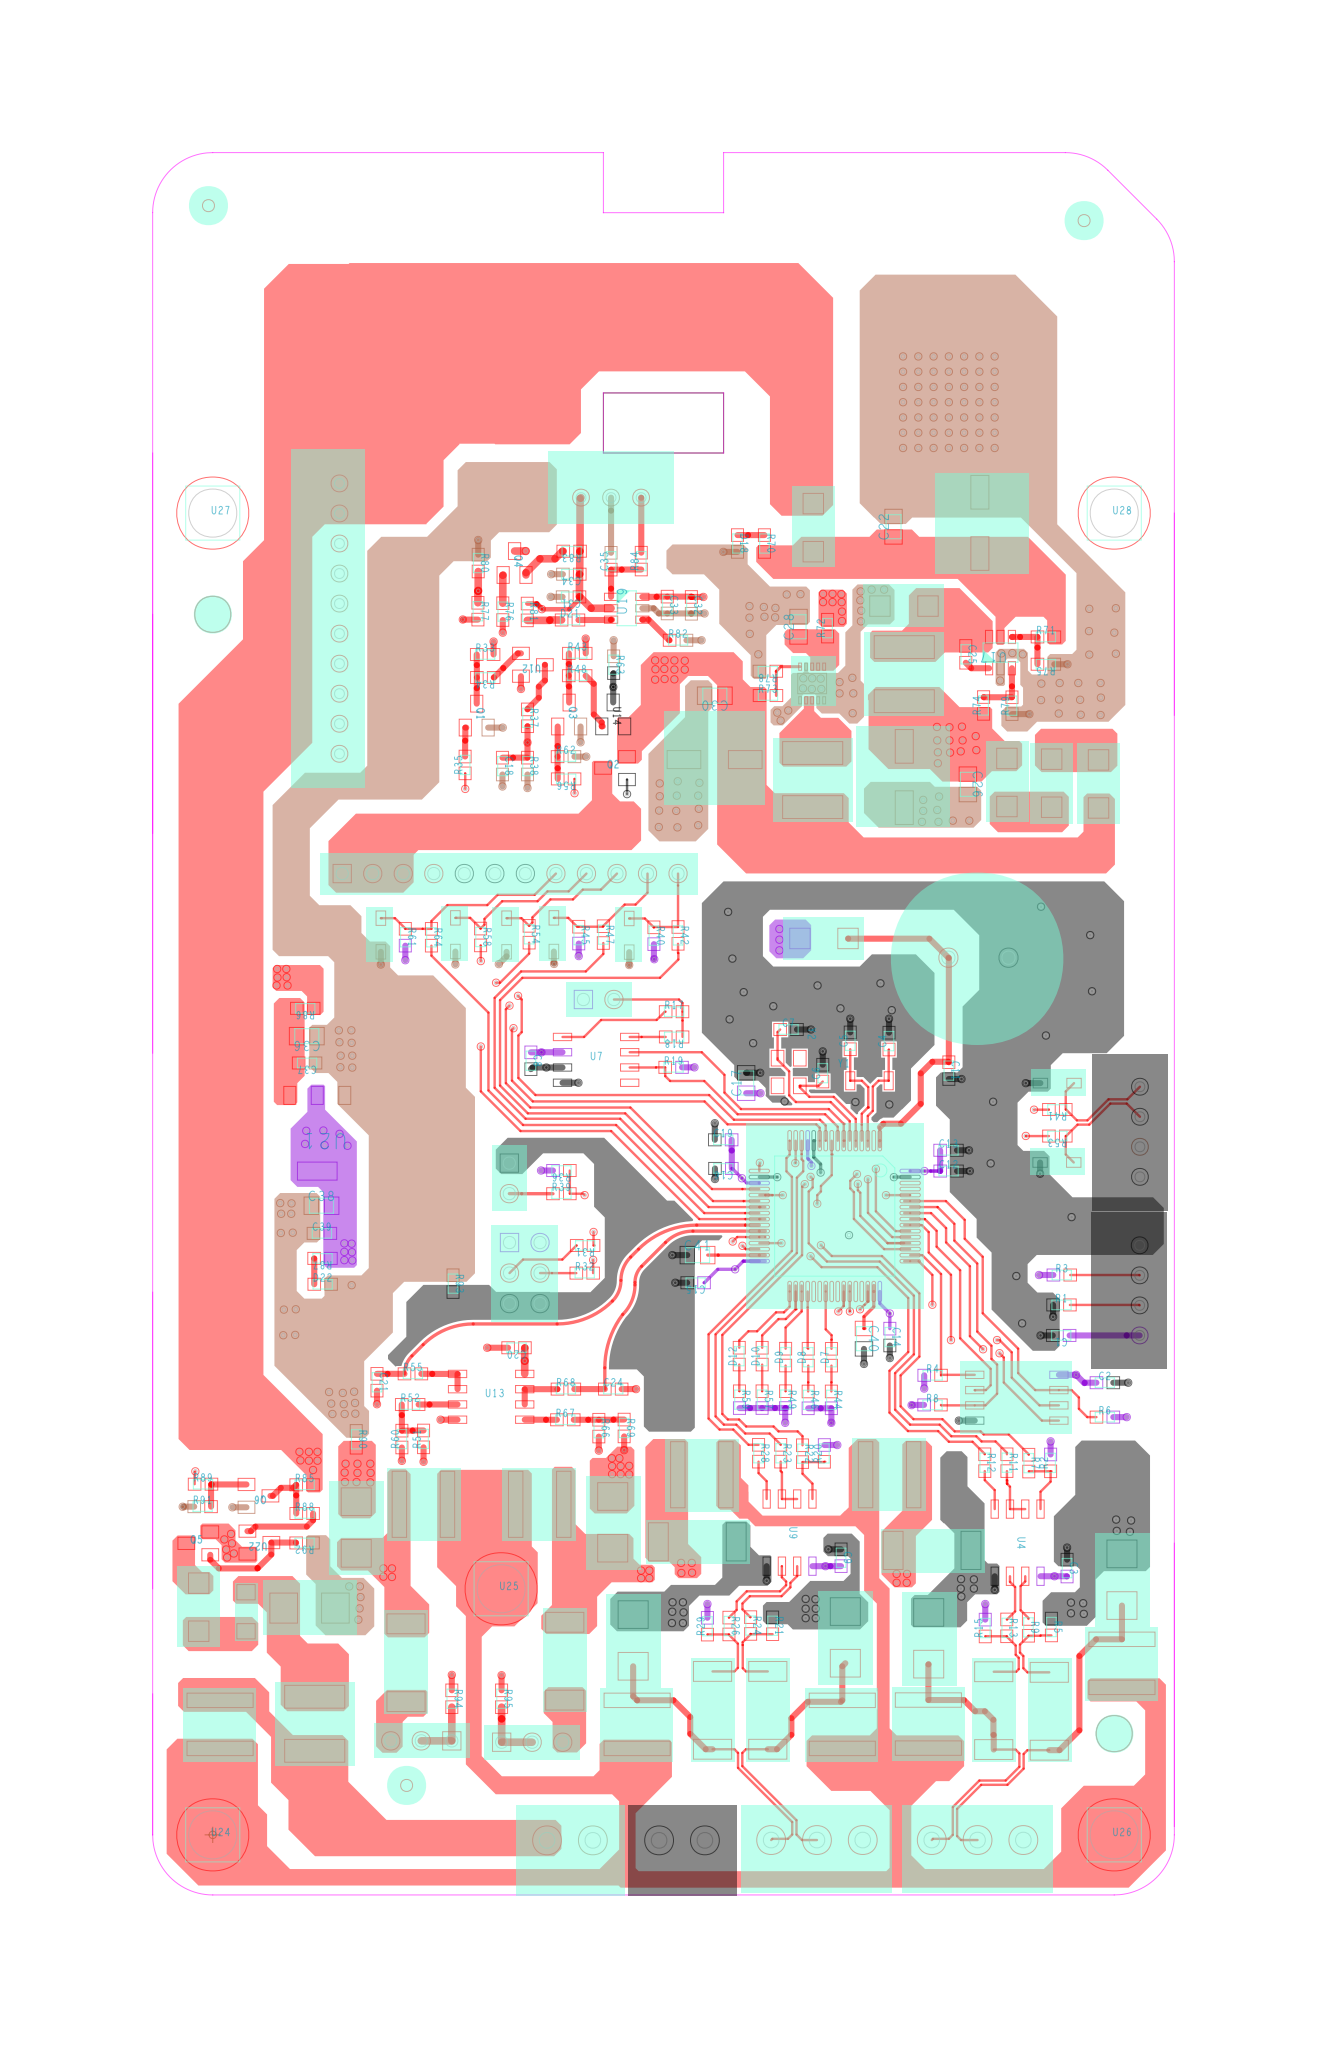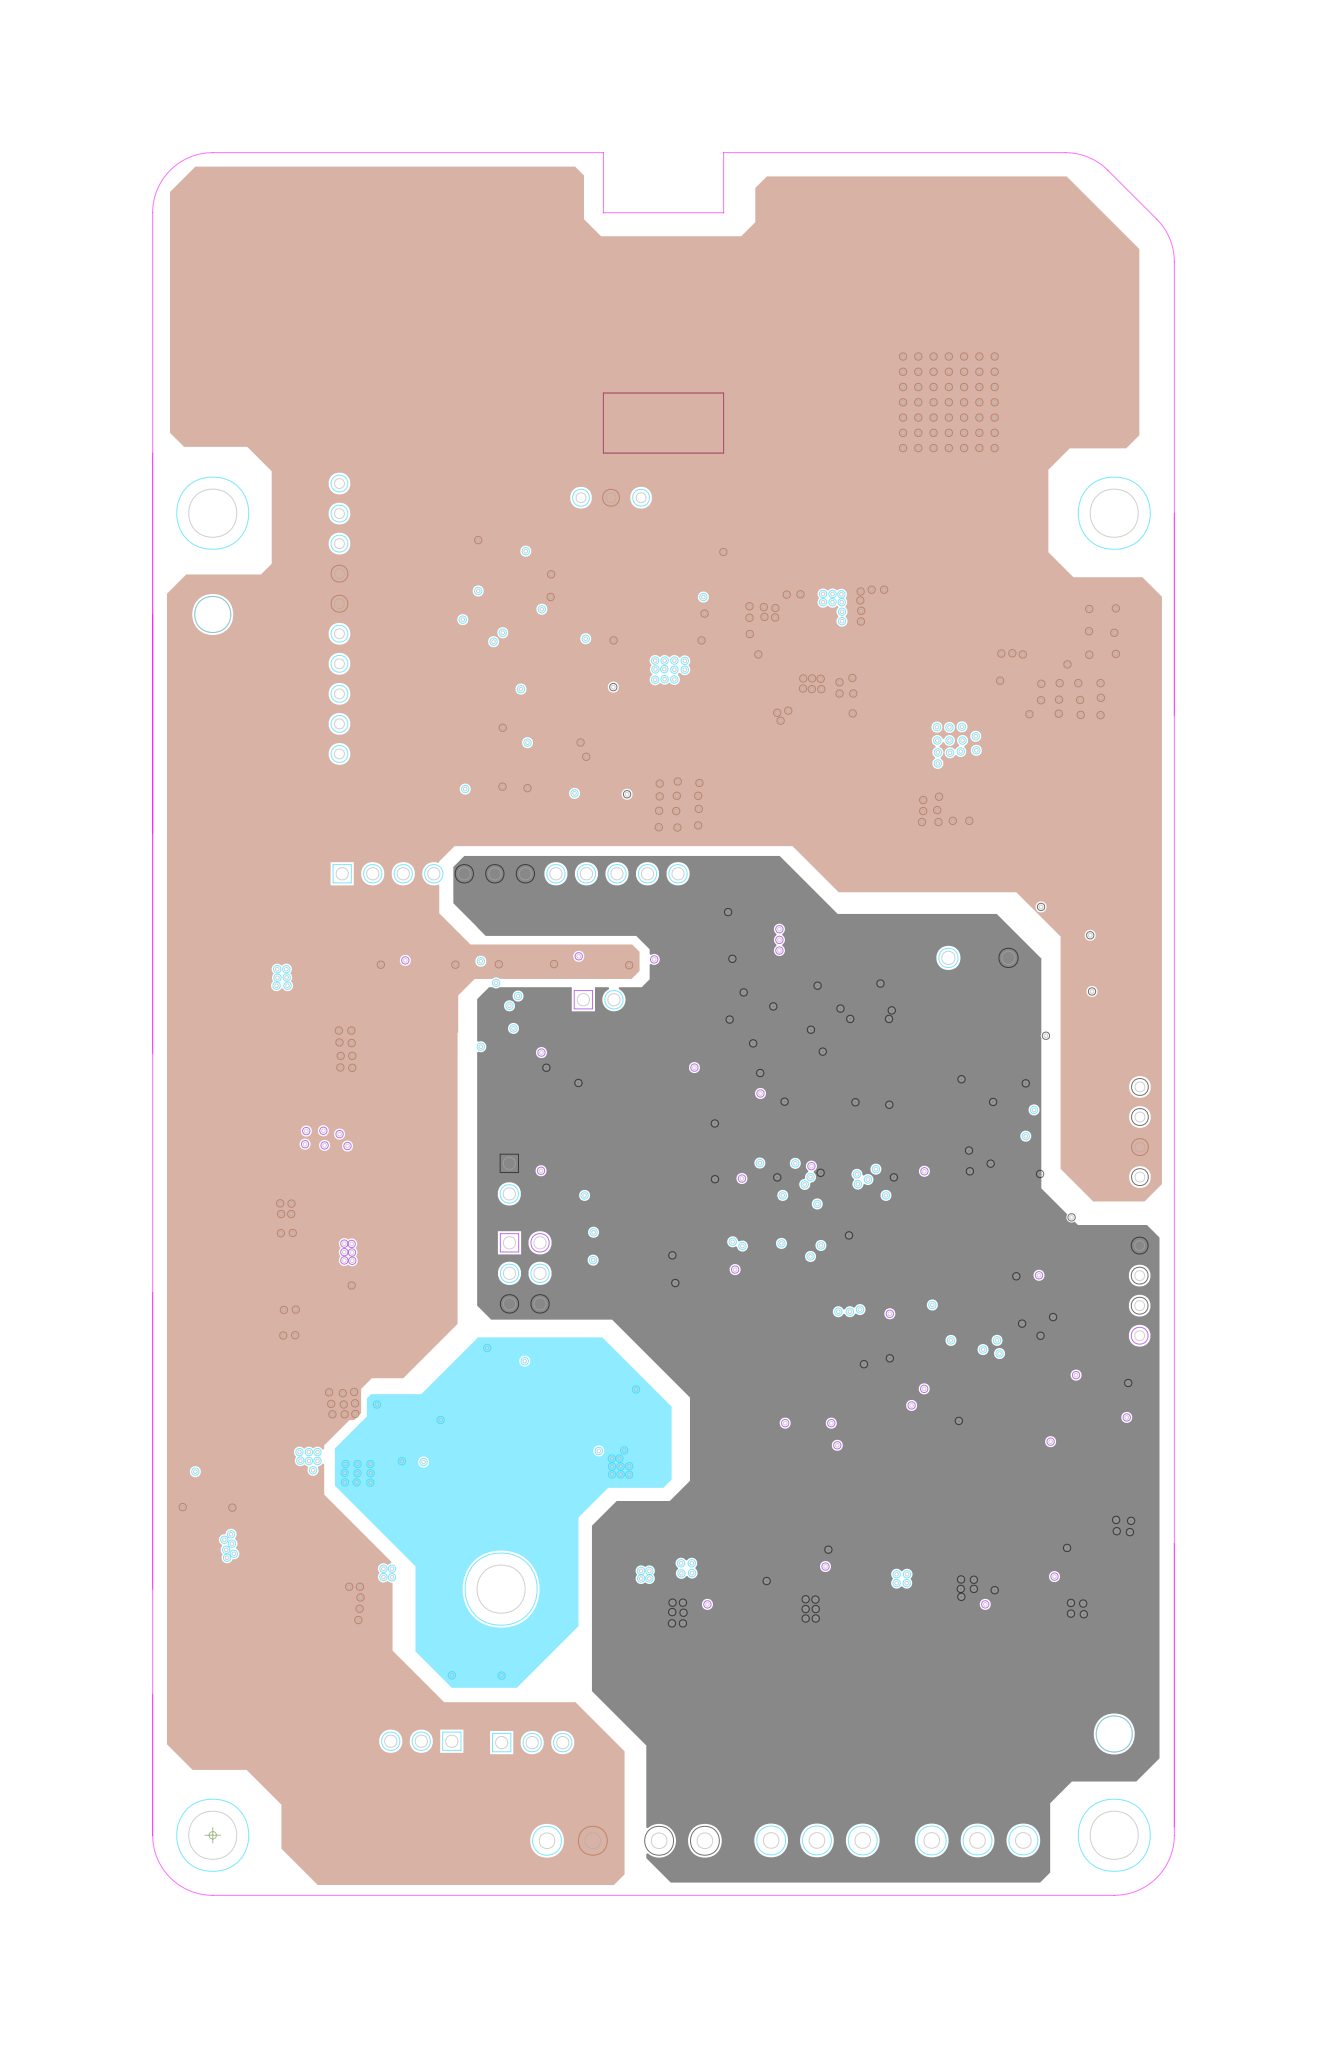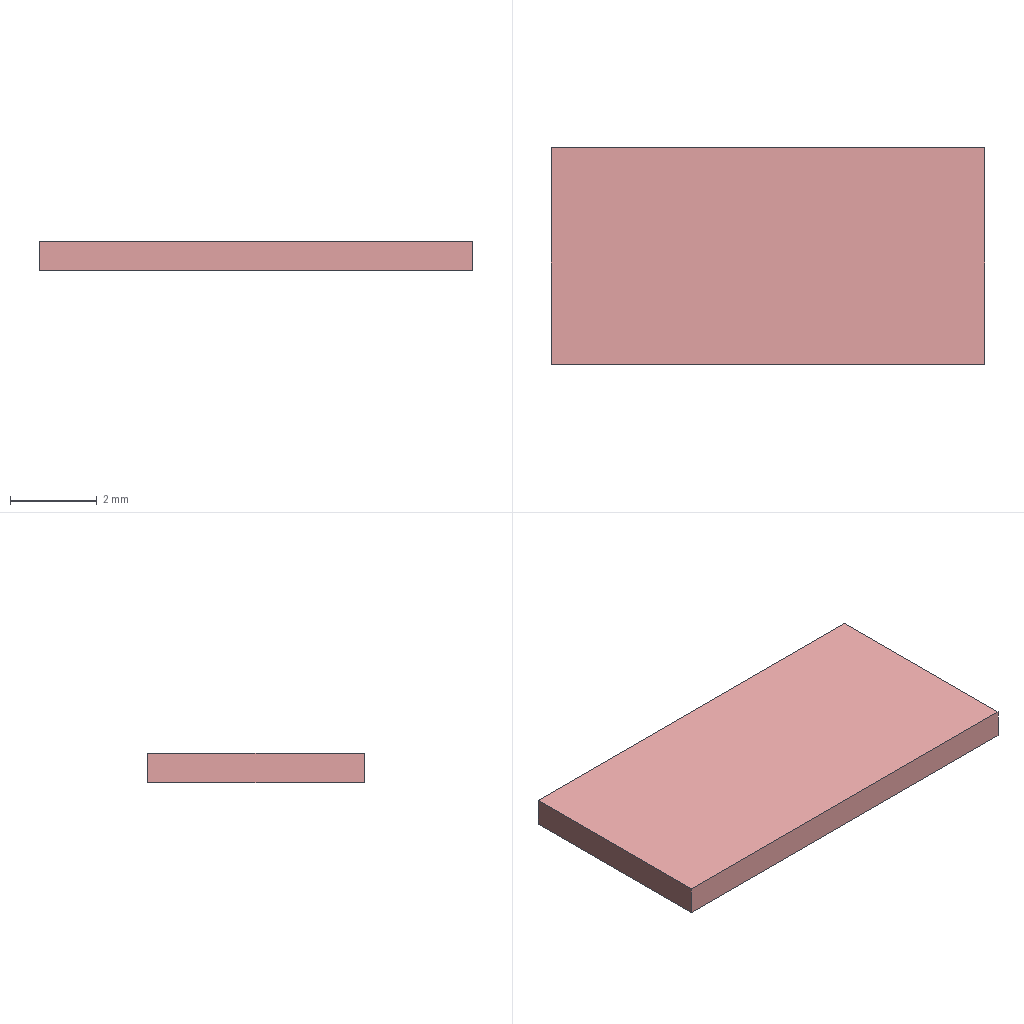Circuit board layout | Cadence Allegro | box 10 x 5 x 0.7 mm
Layer stack:
# Cadence Allegro layer stack of  (unit mm; from the constraint file cross-section; dielectric type: 0 not recorded (Allegro does not mark core vs prepreg), 3 surface material)
index,name,kind,layer,copper_thickness_mm,dielectric_type,dielectric_thickness_mm,dielectric_material,dielectric_constant
0,Top Surface,other,,,,,,
1,TOP,copper,TOP,0.0305,,,,
2,Dielectric1,dielectric,,,0,0.2032,FR-4,4.5
3,GND02,copper,GND02,0.0305,,,,
4,Dielectric2,dielectric,,,0,0.2032,FR-4,4.5
5,PWR03,copper,PWR03,0.0305,,,,
6,Dielectric3,dielectric,,,0,0.2032,FR-4,4.5
7,BOTTOM,copper,BOTTOM,0.0305,,,,
8,Bottom Surface,other,,,,,,
# drill layer pairs: low layer,high layer
drill_pair,TOP,BOTTOM
Part placement:
REFDES,COMP_VALUE,SYM_NAME,SYM_X,SYM_Y,SYM_ROTATE,SYM_MIRROR
C1,104,0603C,2778.984,1636.303,180.000,NO
C2,0.1uF,0603C,2922.020,1481.480,0.000,NO
C3,104,0603C,2798.244,874.031,270.000,NO
C4,22pF,0603C,2215.016,2600.697,90.000,NO
C5,22pF,0603C,2088.016,2601.697,90.000,NO
C6,22pF,0603C,1998.016,2495.697,90.000,NO
C7,22pF,0603C,1886.016,2638.697,0.000,NO
C8,0.1uF,0603C,1042.004,2536.331,270.000,NO
C9,104,0603C,2058.000,908.000,270.000,NO
C10,5.5V/0.47F,FL,2508.000,2874.000,90.000,NO
C11,0.1uF,0603C,2411.000,2504.000,270.000,NO
C12,104,0603C,2410.240,2174.925,0.000,NO
C13,104,0603C,2410.000,2243.000,0.000,NO
C14,104,0603C,2217.717,1630.980,270.000,NO
C15,104,0603C,1581.630,1808.996,180.000,NO
C16,104,0603C,1672.579,2183.469,180.000,NO
C17,2.2uF,0805C,1747.157,2463.398,90.000,NO
C18,0.1uF,0603C,948.925,3501.768,270.000,NO
C19,0.1uF,0603C,1671.984,2277.303,0.000,NO
C20,104,0603C,995.000,1596.000,180.000,NO
C21,104,0603C,537.925,1482.988,270.000,NO
C22,10uF/25V,0805C,2229.819,4286.079,90.000,NO
C23,10uF/25V,F80,2512.614,4298.594,0.000,NO
C24,104,0603C,1311.760,1460.531,0.000,NO
C25,10nF,0603C,2466.480,3867.921,270.000,NO
C26,22uF/10V,0805C,2473.323,3441.937,270.000,NO
C27,10uF/25V,F80,2265.000,3466.000,180.000,NO
C28,22uF,0805C,1918.709,3958.315,90.000,NO
C29,10uF/25V,F80,1643.787,3523.028,90.000,NO
C30,22uF,0805C,1644.429,3732.390,180.000,NO
C31,1uF,0603C,1173.587,4056.232,180.000,NO
C32,0.1uF,0603C,1567.768,4028.409,270.000,NO
C33,1uF,0603C,1488.768,4029.413,270.000,NO
C34,0.1uF,0603C,1174.571,4130.469,180.000,NO
C35,0.1uF,0603C,1304.602,4173.008,90.000,NO
C36,10uF,0805C,308.000,2617.000,180.000,NO
C37,0.1uF,0603C,309.000,2529.000,180.000,NO
C38,10uF,0805C,356.142,2061.291,0.000,NO
C39,0.1uF,0603C,357.492,1970.685,0.000,NO
C40,2.2uF/6.3V,0805C,2133.016,1625.697,270.000,NO
C41,2.2uF/6.3V,0805C,1587.803,1899.524,0.000,NO
D1,SMBJ6.5CA,SMB,2978.000,836.000,270.000,NO
D2,SMBJ6.5CA,SMB,2345.000,644.000,270.000,NO
D3,SMBJ6.5CA,SMB,2072.000,647.000,270.000,NO
D4,30V,SMA,2002.000,2937.000,0.000,NO
D5,SMBJ6.5CA,SMB,1377.000,637.000,270.000,NO
D6,AC,SOD-323,2766.000,2463.000,0.000,NO
D7,LED,LED0603,2026.551,1564.972,90.000,NO
D8,LED,LED0603,1950.551,1565.083,90.000,NO
D9,LED,LED0603,1876.315,1565.303,90.000,NO
D10,LED,LED0603,1799.551,1568.421,90.000,NO
D11,AC,SOD-323,2765.000,2203.000,0.000,NO
D12,LED,LED0603,1724.551,1568.531,90.000,NO
D13,SMBJ15CA,SMB,470.000,1007.000,270.000,NO
D14,SK36,SMA,2264.000,4026.000,0.000,NO
D15,M7,SMA,1967.000,4283.000,270.000,NO
D16,SMBJ15CA,SMB,1310.000,1024.000,270.000,NO
D17,SS36,SMA,2601.244,3448.035,270.000,NO
D18,LED,LED0603,1718.768,4231.071,270.000,NO
D19,SS36,SMA,2747.787,3445.740,90.000,NO
D20,SS36,SMA,2901.244,3443.272,270.000,NO
D21,LED,LED0603,1170.193,3980.449,0.000,NO
D22,LED,LED0603,360.000,1804.000,0.000,NO
D23,M7,SMA,-46.000,746.000,270.000,NO
D24,SMBJ15CA,SMB,317.000,743.000,0.000,NO
D25,AC,SOD323,794.764,2949.346,90.000,NO
D26,AC,SOD323,550.583,2948.346,90.000,NO
D27,AC,SOD323,962.461,2948.346,90.000,NO
D28,AC,SOD323,1117.280,2949.346,90.000,NO
D29,AC,SOD323,1364.098,2947.346,90.000,NO
F1,JK-NSMD010,1206,109.000,731.000,270.000,NO
J1,USB,XR1X4,3036.000,1784.000,90.000,NO
J2,down,DIP2X1,1264.000,2737.000,90.000,NO
J3,BOOT,DIP2X3,1022.016,1840.697,90.000,NO
J4,485_1,KF2EDG-3_81-3-V,2505.000,-17.000,180.000,NO
J5,485_2,KF2EDG-3_81-3-V,1979.000,-17.000,180.000,NO
J6,CON2,KF2EDG-3_81-2-V,1170.000,-18.000,180.000,NO
J7,CON2,KF2EDG-3_81-2-V,1537.000,-18.000,180.000,NO
J8,SYS_RST,DIP2X1,971.346,2150.925,0.000,NO
J9,CON10,XR1X10,415.000,3985.000,90.000,NO
J10,USB,XR1X4,3036.890,2303.563,90.000,NO
J11,CON12,DIP1X12,974.016,3149.606,90.000,NO
J12,JUM1,DIP1X3,1046.323,303.583,90.000,NO
J13,JUM2,DIP1X3,683.000,308.000,270.000,NO
L1,SLF7032T-6R8M1R6-2PF,6045,2265.000,3803.000,270.000,NO
L2,INDUCTOR,6045,1965.000,3456.000,270.000,NO
L3,SMTDR32-560M,6045,334.000,364.000,90.000,NO
Q1,NPN,SOT-23,864.531,3666.685,270.000,NO
Q2,PMOS-3P,SOT-23,1318.000,3495.000,0.000,NO
Q3,NPN,SOT-23,1167.240,3670.295,270.000,NO
Q4,PMOS-3P,SOT-23,988.531,4166.685,270.000,NO
Q5,PMOS-3P,SOT-23,-47.000,955.000,0.000,NO
Q6,NPN,SOT-23,149.295,1110.760,180.000,NO
R1,10k,0603R,2779.984,1736.303,0.000,NO
R2,4.7k,0603R,2744.315,1218.780,90.000,NO
R3,10k,0603R,2780.984,1834.303,0.000,NO
R4,10k,0603R,2357.866,1505.717,0.000,NO
R5,4.7k,0603R,2747.000,681.000,270.000,NO
R6,10k,0603R,2922.087,1368.717,0.000,NO
R7,330,0603R,2672.717,1217.945,270.000,NO
R8,10k,0603R,2357.528,1408.717,0.000,NO
R9,330,0603R,2671.717,679.835,270.000,NO
R10,5.1/2W,2512,2740.000,405.000,270.000,NO
R11,330,0603R,2601.244,1219.370,270.000,NO
R12,330,0603R,2528.717,1219.374,270.000,NO
R13,330,0603R,2600.717,678.264,270.000,NO
R14,5.1/2W,2512,2558.000,407.000,270.000,NO
R15,4.7k,0603R,2530.315,677.669,90.000,NO
R16,5.1/2W,2512,2356.000,932.000,180.000,NO
R17,2k,0603R,1511.000,2697.000,0.000,NO
R18,2k,0603R,1511.228,2614.315,180.000,NO
R19,2k,0603R,1509.488,2514.717,0.000,NO
R20,4.7k,0603R,2003.315,1249.780,90.000,NO
R21,4.7k,0603R,1833.717,685.063,270.000,NO
R22,330,0603R,1931.717,1248.945,270.000,NO
R23,330,0603R,1860.244,1250.370,270.000,NO
R24,330,0603R,1761.717,685.835,270.000,NO
R25,5.1/2W,2512,1818.000,408.000,270.000,NO
R26,330,0603R,1690.717,684.264,270.000,NO
R27,5.1/2W,2512,1637.000,408.000,270.000,NO
R28,330,0603R,1787.717,1250.374,270.000,NO
R29,4.7k,0603R,1620.315,683.669,90.000,NO
R30,5.1/2W,2512,1587.000,960.000,180.000,NO
R31,100k,0603R,1219.720,1931.075,180.000,NO
R32,100k,0603R,1218.358,1840.531,0.000,NO
R33,10k,0603R,892.248,3867.398,0.000,NO
R34,10k,0603R,892.673,3791.996,180.000,NO
R35,4.7k,0603R,826.602,3505.539,90.000,NO
R36,10k,0603R,1142.016,2176.697,180.000,NO
R37,12k,0603R,1030.925,3659.949,270.000,NO
R38,30k,0603R,1030.925,3501.839,270.000,NO
R39,330,0603R,1142.016,2100.697,0.000,NO
R40,100k,0603R,1445.000,2946.000,270.000,NO
R41,RES2,0603R,2766.350,2376.531,180.000,NO
R42,330,0603R,1524.000,2947.000,270.000,NO
R43,1k,0603R,1194.000,3871.000,0.000,NO
R44,2k,0603R,2026.244,1425.311,270.000,NO
R45,100k,0603R,1198.756,2947.898,270.000,NO
R46,2k,0603R,1950.244,1425.201,270.000,NO
R47,330,0603R,1279.283,2949.618,270.000,NO
R48,1k,0603R,1193.713,3797.925,0.000,NO
R49,2k,0603R,1876.244,1426.091,270.000,NO
R50,5.1/2W,2512,633.000,564.000,270.000,NO
R51,91k/1%,0603R,690.469,1297.339,90.000,NO
R52,10k,0603R,646.657,1410.004,0.000,NO
R53,RES2,0603R,2766.461,2289.531,180.000,NO
R54,330,0603R,1036.283,2950.728,270.000,NO
R55,100,0603R,655.559,1510.531,0.000,NO
R56,1k,0603R,1157.496,3459.787,180.000,NO
R57,2k,0603R,1799.244,1425.980,270.000,NO
R58,330,0603R,877.283,2941.839,270.000,NO
R59,2k,0603R,1725.244,1425.870,270.000,NO
R60,30k/1%,0603R,619.469,1296.780,90.000,NO
R61,100k,0603R,630.756,2941.008,270.000,NO
R62,4.7k,0603R,1157.047,3532.717,0.000,NO
R63,100k,0603R,1313.000,3834.000,270.000,NO
R64,330,0603R,716.283,2940.949,270.000,NO
R65,5.1/2W,2512,1153.000,569.000,270.000,NO
R66,91k/1%,0603R,1264.531,1332.551,270.000,NO
R67,10k,0603R,1154.878,1360.004,0.000,NO
R68,100,0603R,1156.669,1460.531,0.000,NO
R69,30k/1%,0603R,1347.531,1333.110,270.000,NO
R70,10k,0603R,1807.004,4231.012,270.000,NO
R71,100k,0603R,2728.941,3924.925,0.000,NO
R72,0,0603R,2013.787,3953.713,90.000,NO
R73,536k/1%,0603R,1818.583,3732.925,0.000,NO
R74,49.9k/1%,0603R,2524.787,3700.374,90.000,NO
R75,30k,0603R,2728.760,3835.469,180.000,NO
R76,10k,0603R,950.004,4007.902,270.000,NO
R77,2.74K/1%,0603R,868.531,4009.228,270.000,NO
R78,100k/1%,0603R,1818.118,3812.469,180.000,NO
R79,9.53k/1%,0603R,2617.787,3699.701,90.000,NO
R80,4.7K/1%,0603R,869.531,4166.902,270.000,NO
R81,2k,0603R,1030.244,4006.760,270.000,NO
R82,2k,0603R,1524.000,3914.000,0.000,NO
R83,0,0603R,1175.571,4205.756,180.000,NO
R84,10k,0603R,1403.602,4173.350,90.000,NO
R85,1k,0603R,300.933,1146.925,0.000,NO
R86,0,0603R,303.000,2708.000,180.000,NO
R87,2k,0603R,359.539,1888.756,180.000,NO
R88,1k,0603R,301.043,1052.925,0.000,NO
R89,1k,0603R,-31.850,1148.925,0.000,NO
R90,0,0603R,470.000,1296.000,270.000,NO
R91,4.7k,0603R,-33.130,1075.398,0.000,NO
R92,1k,0603R,300.772,956.469,180.000,NO
R93,0,0603R,787.000,1806.000,270.000,NO
R94,249/1%,0603R,783.000,446.000,270.000,NO
R95,249/1%,0603R,946.000,446.000,270.000,NO
U1,STM32F205,LQFP-64,2037.244,2027.366,270.000,NO
U2,25Q32VSIG,SOIC-8_208,2633.634,1432.244,0.000,NO
U3,470M,SMD5050,2978.000,562.000,270.000,NO
U4,SP3485E,SO8,2711.244,1067.366,270.000,NO
U5,470M,SMD5050,2344.000,363.000,270.000,NO
U6,470M,SMD5050,2217.000,1180.000,180.000,NO
U7,MAX706R,SO8,1145.634,2614.244,0.000,NO
U8,470M,SMD5050,2062.000,362.000,270.000,NO
U9,SP3485E,SO8,1964.244,1100.366,270.000,NO
U10,470M,SMD5050,1602.000,1180.000,0.000,NO
U11,470M,SMD5050,1390.000,362.000,270.000,NO
U12,PNP,SOT-23,1048.295,3833.760,180.000,NO
U13,LM2904,SO8,801.854,1510.240,0.000,NO
U14,PNP,SOT-23,1311.531,3670.685,270.000,NO
U15,470M,SMD5050,690.000,1083.000,0.000,NO
U16,470M,SMD5050,1071.000,1083.000,180.000,NO
U17,MP2359DJ,SOT23-6,2580.181,3873.598,90.000,NO
U18,SGM6014ADJ,TDFN-3X3-10L,1963.244,3772.366,270.000,NO
U19,BQ21040,SOT23-6,1355.850,4018.850,0.000,NO
U20,BAT,XR1X3,1304.618,4381.417,0.000,NO
U21,TLV1117LV,SOT-223,432.366,2422.756,180.000,NO
U22,PNP,SOT-23,152.295,957.760,180.000,NO
U23,470M,SMD5050,24.000,362.000,270.000,NO
U24,TEST POINT A,HOLE,0.000,0.000,0.000,NO
U25,TEST POINT A,HOLE,944.531,806.287,0.000,NO
U26,TEST POINT A,HOLE,2952.756,0.000,0.000,NO
U27,TEST POINT A,HOLE,0.000,4330.709,0.000,NO
U28,TEST POINT A,HOLE,2952.756,4330.709,0.000,NO
Y1,8M,XTAL3215,2088.016,2470.697,0.000,NO
Y2,32.768K,XTAL3225,1850.016,2544.697,270.000,NO
Pad and via stacks:
# Allegro (Cadence) via spans and padstacks; design units: ("mils" 3 1000)
# via spans: padstack,start_layer,end_layer,net_example,count
VIA12_24,ETCH/TOP,ETCH/BOTTOM,VCC_12V,435
# Allegro padstack definitions: name,start_layer,end_layer,drill,plating,holeType,type
VIA30D16,"ETCH/TOP","ETCH/BOTTOM",16.0,"PLATED","circle_drill","through"
R180_160,"ETCH/TOP","ETCH/TOP",0.0,"PLATED","none","smd"
PTH_C472D276S40,"ETCH/TOP","ETCH/BOTTOM",27.559,"PLATED","circle_drill","through"
PTH_S472D276S40,"ETCH/TOP","ETCH/BOTTOM",27.559,"PLATED","circle_drill","through"
RE118_11X98_43,"ETCH/TOP","ETCH/TOP",0.0,"NON_PLATED","none","smd"
C43_31D43_31,"ETCH/TOP","ETCH/BOTTOM",43.311,"PLATED","circle_drill","through"
R105_100,"ETCH/TOP","ETCH/TOP",0.0,"PLATED","none","smd"
R170_135,"ETCH/TOP","ETCH/TOP",0.0,"PLATED","none","smd"
R145_120,"ETCH/TOP","ETCH/TOP",0.0,"PLATED","none","smd"
RE350X100,"ETCH/TOP","ETCH/TOP",0.0,"PLATED","none","smd"
RE55X40,"ETCH/TOP","ETCH/TOP",0.0,"NON_PLATED","none","smd"
R225_160,"ETCH/TOP","ETCH/TOP",0.0,"PLATED","none","smd"
S210,"ETCH/TOP","ETCH/TOP",0.0,"PLATED","none","smd"
RE90X95,"ETCH/TOP","ETCH/TOP",0.0,"NON_PLATED","none","smd"
SMD_R787X1181P0S40,"ETCH/TOP","ETCH/TOP",0.0,"PLATED","none","smd"
SMD_R98X472P0S40,"ETCH/TOP","ETCH/TOP",0.0,"PLATED","none","smd"
S220H120T220_240_40,"ETCH/TOP","ETCH/BOTTOM",47.244,"PLATED","circle_drill","through"
C220H120T220_240_40,"ETCH/TOP","ETCH/BOTTOM",47.244,"PLATED","circle_drill","through"
S160H105T155_190_40,"ETCH/TOP","ETCH/BOTTOM",41.339,"PLATED","circle_drill","through"
C160H105T155_190_40,"ETCH/TOP","ETCH/BOTTOM",41.339,"PLATED","circle_drill","through"
SMD_R472X709P0S40,"ETCH/TOP","ETCH/TOP",0.0,"PLATED","none","smd"
SMD_R276X709P0S40,"ETCH/TOP","ETCH/TOP",0.0,"PLATED","none","smd"
SMD_R591X1102P0S40,"ETCH/TOP","ETCH/TOP",0.0,"PLATED","none","smd"
SMD_R433X709P0S40,"ETCH/TOP","ETCH/TOP",0.0,"PLATED","none","smd"
PTH_O1800X800SLOT500X1100S40,"ETCH/TOP","ETCH/BOTTOM",50.0,"PLATED","oval slot","through"
PTH_O800X1800SLOT500X1200S40,"ETCH/TOP","ETCH/BOTTOM",50.0,"PLATED","oval slot","through"
PTH_O800X1800SLOT500X1100S40,"ETCH/TOP","ETCH/BOTTOM",50.0,"PLATED","oval slot","through"
PTH_S630D362S40,"ETCH/TOP","ETCH/BOTTOM",36.22,"PLATED","circle_drill","through"
PTH_C630D362S40,"ETCH/TOP","ETCH/BOTTOM",36.22,"PLATED","circle_drill","through"
PTH_C1496D906S40,"ETCH/TOP","ETCH/BOTTOM",90.551,"PLATED","circle_drill","through"
SMD_R984X787P0S40,"ETCH/TOP","ETCH/TOP",0.0,"PLATED","none","smd"
SMD_R236X787P0S40,"ETCH/TOP","ETCH/TOP",0.0,"PLATED","none","smd"
S140H80,"ETCH/TOP","ETCH/BOTTOM",31.496,"PLATED","circle_drill","through"
C140H80,"ETCH/TOP","ETCH/BOTTOM",31.496,"PLATED","circle_drill","through"
S140H90T140_170_40,"ETCH/TOP","ETCH/BOTTOM",35.433,"PLATED","circle_drill","through"
C140H90T140_170_40,"ETCH/TOP","ETCH/BOTTOM",35.433,"PLATED","circle_drill","through"
C355H235T285_330_50,"ETCH/TOP","ETCH/BOTTOM",92.52,"PLATED","circle_drill","through"
PTH_C591D402S40,"ETCH/TOP","ETCH/BOTTOM",40.161,"PLATED","circle_drill","through"
PTH_C600D350S40,"ETCH/TOP","ETCH/BOTTOM",35.0,"PLATED","circle_drill","through"
PTH_C866D650S40,"ETCH/TOP","ETCH/BOTTOM",64.961,"PLATED","circle_drill","through"
PTH_S600D350S40,"ETCH/TOP","ETCH/BOTTOM",35.0,"PLATED","circle_drill","through"
RE200X125,"ETCH/TOP","ETCH/TOP",0.0,"PLATED","none","smd"
RE75X40,"ETCH/TOP","ETCH/TOP",0.0,"NON_PLATED","none","smd"
SQ120,"ETCH/TOP","ETCH/TOP",0.0,"PLATED","none","smd"
RE620X580,"ETCH/TOP","ETCH/TOP",0.0,"NON_PLATED","none","smd"
RE300X160,"ETCH/TOP","ETCH/TOP",0.0,"NON_PLATED","none","smd"
C100H60,"ETCH/TOP","ETCH/BOTTOM",23.622,"PLATED","circle_drill","through"
RE100H60,"ETCH/TOP","ETCH/BOTTOM",23.622,"PLATED","circle_drill","through"
R105_45,"ETCH/TOP","ETCH/TOP",0.0,"PLATED","none","smd"
RE65X180,"ETCH/TOP","ETCH/TOP",0.0,"PLATED","none","smd"
H70,"ETCH/TOP","ETCH/BOTTOM",27.559,"PLATED","circle_drill","through"
SMD_R100X650P0S40,"ETCH/TOP","ETCH/TOP",0.0,"PLATED","none","smd"
RE150X80,"ETCH/TOP","ETCH/TOP",0.0,"NON_PLATED","none","smd"
SMD_R512X413P0S40,"ETCH/TOP","ETCH/TOP",0.0,"PLATED","none","smd"
RE60X24,"ETCH/TOP","ETCH/TOP",0.0,"NON_PLATED","none","smd"
RE43_31X19_68,"ETCH/TOP","ETCH/TOP",0.0,"PLATED","none","smd"
RE134X170,"ETCH/TOP","ETCH/TOP",0.0,"PLATED","none","smd"
R110_60,"ETCH/TOP","ETCH/TOP",0.0,"PLATED","none","smd"
RE100X150,"ETCH/TOP","ETCH/TOP",0.0,"PLATED","none","smd"
RE330X150,"ETCH/TOP","ETCH/TOP",0.0,"PLATED","none","smd"
RE39_37X11_81,"ETCH/TOP","ETCH/TOP",0.0,"NON_PLATED","none","smd"
RE11_81X39_37,"ETCH/TOP","ETCH/TOP",0.0,"NON_PLATED","none","smd"
SQ124,"ETCH/TOP","ETCH/TOP",0.0,"NON_PLATED","none","smd"
SQ20,"ETCH/TOP","ETCH/TOP",0.0,"NON_PLATED","none","smd"
R155_60,"ETCH/TOP","ETCH/TOP",0.0,"PLATED","none","smd"
SMD_R118X315P0S40,"ETCH/TOP","ETCH/TOP",0.0,"PLATED","none","smd"
R27X39,"ETCH/TOP","ETCH/TOP",0.0,"PLATED","none","smd"
SMD_R98X315P0S40,"ETCH/TOP","ETCH/TOP",0.0,"PLATED","none","smd"
SMD_S984P0S40,"ETCH/TOP","ETCH/TOP",0.0,"PLATED","none","smd"
SMD_R591X295P0S40,"ETCH/TOP","ETCH/TOP",0.0,"PLATED","none","smd"
SMD_R295X591P0S40,"ETCH/TOP","ETCH/TOP",0.0,"PLATED","none","smd"
PTH_C600D300S40,"ETCH/TOP","ETCH/BOTTOM",30.0,"PLATED","circle_drill","through"
C177_17D137_80,"ETCH/TOP","ETCH/BOTTOM",157.48,"PLATED","circle_drill","through"
B160_60,"ETCH/TOP","ETCH/TOP",0.0,"PLATED","none","smd"
PTH_O1024X709SLOT394X630S40,"ETCH/TOP","ETCH/BOTTOM",39.37,"PLATED","oval slot","through"
VIA12_24,"ETCH/TOP","ETCH/BOTTOM",12.0,"PLATED","circle_drill","through"
Y300,"ETCH/TOP","ETCH/BOTTOM",118.11,"NON_PLATED","circle_drill","through"
C83D53,"ETCH/TOP","ETCH/BOTTOM",53.0,"PLATED","circle_drill","through"
R18X20,"ETCH/TOP","ETCH/TOP",0.0,"NON_PLATED","none","smd"
Y3,"ETCH/TOP","ETCH/TOP",0.0,"PLATED","none","smd"
SMD_OV65X12,"ETCH/TOP","ETCH/TOP",0.0,"PLATED","none","smd"
F15,"ETCH/TOP","ETCH/BOTTOM",40.0,"PLATED","circle_drill","through"
F152,"ETCH/TOP","ETCH/BOTTOM",40.0,"PLATED","circle_drill","through"
R23X25,"ETCH/TOP","ETCH/TOP",0.0,"NON_PLATED","none","smd"
S17,"ETCH/TOP","ETCH/TOP",0.0,"NON_PLATED","none","smd"
R12X8,"ETCH/TOP","ETCH/TOP",0.0,"NON_PLATED","none","smd"
R127X152,"ETCH/TOP","ETCH/TOP",0.0,"NON_PLATED","none","smd"
R50X30,"ETCH/TOP","ETCH/TOP",0.0,"NON_PLATED","none","smd"
R35X16,"ETCH/TOP","ETCH/TOP",0.0,"PLATED","none","smd"
Y6T,"ETCH/TOP","ETCH/BOTTOM",43.307,"PLATED","circle_drill","through"
Y8T,"ETCH/TOP","ETCH/BOTTOM",32.283,"PLATED","circle_drill","through"
R15X28,"ETCH/TOP","ETCH/TOP",0.0,"NON_PLATED","none","smd"
Y24,"ETCH/TOP","ETCH/BOTTOM",51.181,"PLATED","circle_drill","through"
R60X24,"ETCH/TOP","ETCH/TOP",0.0,"PLATED","none","smd"
R170X240,"ETCH/TOP","ETCH/TOP",0.0,"PLATED","none","smd"
D3,"ETCH/TOP","ETCH/BOTTOM",118.11,"NON_PLATED","circle_drill","through"
R550X120,"ETCH/TOP","ETCH/TOP",0.0,"PLATED","none","smd"
R500X190,"ETCH/TOP","ETCH/TOP",0.0,"PLATED","none","smd"
R165X317,"ETCH/TOP","ETCH/TOP",0.0,"NON_PLATED","none","smd"
Design rules, without the lines most boards share, first 13 of 25 lines:
# Cadence Allegro design rules of  (from the Constraint Manager export constraints.dcfx, design unit mil; typed fields in mm)
# columns: name | kind | enabled | priority | scope1 | scope2 | descriptor | typed fields (field=value)
# Allegro precedence (priority 1 wins): 1 Region class-to-class, 2 Region class, 3 Region, 4 class-to-class, 5 DiffPair/Bus/NetGroup override, 6 NetClass, 7 constraint set (CSet) default
# per-layer values are written LAYER=value in the descriptor and LAYER:mm in the typed field; a maximum of 0 means no limit set
# --- net classes (and buses / net groups) ---
# (no net classes defined: every net uses the default constraint sets)
# --- track widths, neck and differential-pair gap (physical constraint sets) ---
DEFAULT | PhysicalCSet | enabled | 7 | Design default | All | Physical Constraint (Min Line Width=8mil) (Max Line Width=100mil) (Min Neck Width=6mil) (Max Neck Length=6mil) (DiffPair Primary Gap=6mil) (DiffPair Neck Gap=6mil) (DiffPair Min Space=6mil) (DiffPair Coupled +Tol=6mil) (DiffPair Coupled -Tol=6mil) (Min BB Via Stagger=6mil) (Max BB Via Stagger=6mil) (T-junctions=ANYWHERE) (Pad-pad direct connect=ALL_ALLOWED) (Allowed vias=VIA12_24) | min_line_width=0.2032 min_neck_width=0.1524 min_bvia_stagger=0.1524 max_bvia_stagger=0.1524 ts_allowed=ANYWHERE diffp_primary_gap=0.1524 diffp_neck_gap=0.1524 max_line_width=2.54 maximum_neck_length=0.1524 pad_pad_direct_connect=ALL_ALLOWED allow_on_etch_subclass=TRUE diffp_coupled_plus=0.1524 diffp_coupled_minus=0.1524 diffp_min_space=0.1524 vias=VIA12_24
# --- clearances: line / pad / via / shape / hole (spacing constraint sets) ---
DEFAULT | SpacingCSet | enabled | 7 | Design default | All | Clearance Constraint (Line-Line=6mil) (Line-SMD Pad=8mil) (Line-Thru Pin=8mil) (Line-Via=8mil) (Line-Shape=8mil) (SMD Pad-SMD Pad=7mil) (Thru Pin-Thru Pin=8mil) (Thru Pin-SMD Pad=7mil) (SMD Pad-Via=8mil) (Thru Pin-Via=8mil) (Via-Via=6mil) (Shape-SMD Pad=6mil) (Shape-Thru Pin=8mil) (Shape-Via=6mil) (Shape-Shape=6mil) (Hole-Hole=8mil) (Hole-Line=8mil) (Hole-Shape=8mil) (BB Via-BB Via=6mil) (uVia-uVia=5mil) | thrupin_to_thrupin_spacing=0.2032 thrupin_to_smdpin_spacing=0.1778 thrupin_to_thruvia_spacing=0.2032 line_to_thrupin_spacing=0.2032 thrupin_to_shape_spacing=0.2032 smdpin_to_smdpin_spacing=0.1778 smdpin_to_thruvia_spacing=0.2032 line_to_smdpin_spacing=0.2032 shape_to_smdpin_spacing=0.1524 thruvia_to_thruvia_spacing=0.1524 line_to_thruvia_spacing=0.2032 shape_to_thruvia_spacing=0.1524 line_to_line_spacing=0.1524 line_to_shape_spacing=0.2032 shape_to_shape_spacing=0.1524 bbv_to_bbv_spacing=0.1524 bbv_to_thrupin_spacing=0.2032 bbv_to_smdpin_spacing=0.2032 bbv_to_thruvia_spacing=0.1524 bbv_to_line_spacing=0.2032 bbv_to_shape_spacing=0.1524 bbv_to_testpin_spacing=0.1524 bbv_to_testvia_spacing=0.1524 testpin_to_testpin_spacing=0.1778 testpin_to_thrupin_spacing=0.2032 smdpin_to_testpin_spacing=0.2032 testpin_to_thruvia_spacing=0.1524 testpin_to_testvia_spacing=0.1524 line_to_testpin_spacing=0.2032 shape_to_testpin_spacing=0.1524 testvia_to_testvia_spacing=0.127 testvia_to_thrupin_spacing=0.2032 smdpin_to_testvia_spacing=0.2032 testvia_to_thruvia_spacing=0.1524 line_to_testvia_spacing=0.2032 shape_to_testvia_spacing=0.1524 bondpad_to_bondpad_spacing=0.127 thrupin_to_bondpad_spacing=0.2032 smdpin_to_bondpad_spacing=0.1524 bondpad_to_thruvia_spacing=0.1524 bondpad_to_line_spacing=0.2032 bondpad_to_shape_spacing=0.1524 bondpad_to_bbv_spacing=0.1524 bondpad_to_testpin_spacing=0.1524 bondpad_to_testvia_spacing=0.127 min_bvia_gap=0.127 hole_to_pin_spacing=0.2032 hole_to_via_spacing=0.2032 hole_to_line_spacing=0.2032 hole_to_shape_spacing=0.2032 hole_to_hole_spacing=0.2032 mvia_to_mvia_spacing=0.127 mvia_to_thrupin_spacing=0.2032 mvia_to_smdpin_spacing=0.2032 mvia_to_thruvia_spacing=0.127 mvia_to_bbv_spacing=0.127 mvia_to_line_spacing=0.2032 mvia_to_shape_spacing=0.127 mvia_to_testpin_spacing=0.127 mvia_to_testvia_spacing=0.127 bondpad_to_mvia_spacing=0.127 bondpad_to_bondpad_diffp_spc=0.127
DEFAULT | SameNetSpacingCSet | enabled | 7 | Design default | All | Same-Net Clearance (Line-Line=5mil) (Line-SMD Pad=5mil) (Line-Thru Pin=5mil) (Line-Via=5mil) (Line-Shape=5mil) (SMD Pad-SMD Pad=5mil) (Thru Pin-Thru Pin=5mil) (Thru Pin-SMD Pad=5mil) (SMD Pad-Via=5mil) (Thru Pin-Via=5mil) (Via-Via=5mil) (Shape-SMD Pad=5mil) (Shape-Thru Pin=5mil) (Shape-Via=5mil) (Shape-Shape=5mil) (Hole-Hole=8mil) (Hole-Line=8mil) (Hole-Shape=8mil) (BB Via-BB Via=5mil) (uVia-uVia=5mil) | sn_thrupin_to_thrupin_spacing=0.127 sn_thrupin_to_smdpin_spacing=0.127 sn_thrupin_to_thruvia_spacing=0.127 sn_line_to_thrupin_spacing=0.127 sn_thrupin_to_shape_spacing=0.127 sn_smdpin_to_smdpin_spacing=0.127 sn_smdpin_to_thruvia_spacing=0.127 sn_line_to_smdpin_spacing=0.127 sn_shape_to_smdpin_spacing=0.127 sn_thruvia_to_thruvia_spacing=0.127 sn_line_to_thruvia_spacing=0.127 sn_shape_to_thruvia_spacing=0.127 sn_line_to_line_spacing=0.127 sn_line_to_shape_spacing=0.127 sn_shape_to_shape_spacing=0.127 sn_bbv_to_bbv_spacing=0.127 sn_bbv_to_thrupin_spacing=0.127 sn_bbv_to_smdpin_spacing=0.127 sn_bbv_to_thruvia_spacing=0.127 sn_bbv_to_line_spacing=0.127 sn_bbv_to_shape_spacing=0.127 sn_bbv_to_testpin_spacing=0.127 sn_bbv_to_testvia_spacing=0.127 sn_testpin_to_testpin_spacing=0.127 sn_testpin_to_thrupin_spacing=0.127 sn_smdpin_to_testpin_spacing=0.127 sn_testpin_to_thruvia_spacing=0.127 sn_testpin_to_testvia_spacing=0.127 sn_line_to_testpin_spacing=0.127 sn_shape_to_testpin_spacing=0.127 sn_testvia_to_testvia_spacing=0.127 sn_testvia_to_thrupin_spacing=0.127 sn_smdpin_to_testvia_spacing=0.127 sn_testvia_to_thruvia_spacing=0.127 sn_line_to_testvia_spacing=0.127 sn_shape_to_testvia_spacing=0.127 sn_bondpad_to_bondpad_spacing=0.127 sn_thrupin_to_bondpad_spacing=0.127 sn_smdpin_to_bondpad_spacing=0.127 sn_bondpad_to_thruvia_spacing=0.127 sn_bondpad_to_line_spacing=0.127 sn_bondpad_to_shape_spacing=0.127 sn_bondpad_to_bbv_spacing=0.127 sn_bondpad_to_testpin_spacing=0.127 sn_bondpad_to_testvia_spacing=0.127 same_net=TRUE sn_hole_to_pin_spacing=0.2032 sn_hole_to_via_spacing=0.2032 sn_hole_to_line_spacing=0.2032 sn_hole_to_shape_spacing=0.2032 sn_hole_to_hole_spacing=0.2032 sn_mvia_to_mvia_spacing=0.127 sn_mvia_to_thrupin_spacing=0.127 sn_mvia_to_smdpin_spacing=0.127 sn_mvia_to_thruvia_spacing=0.127 sn_mvia_to_bbv_spacing=0.127 sn_mvia_to_line_spacing=0.127 sn_mvia_to_shape_spacing=0.127 sn_mvia_to_testpin_spacing=0.127 sn_mvia_to_testvia_spacing=0.127 sn_bondpad_to_mvia_spacing=0.127
# --- differential pairs (2) ---
DIFFPAIR1 | DiffPair | enabled | 5 | A2 | B2 | Differential Pair (Primary Gap=6mil) (Min Line Width=8mil) (Physical CSet=DEFAULT) | gap=0.1524 width=0.2032